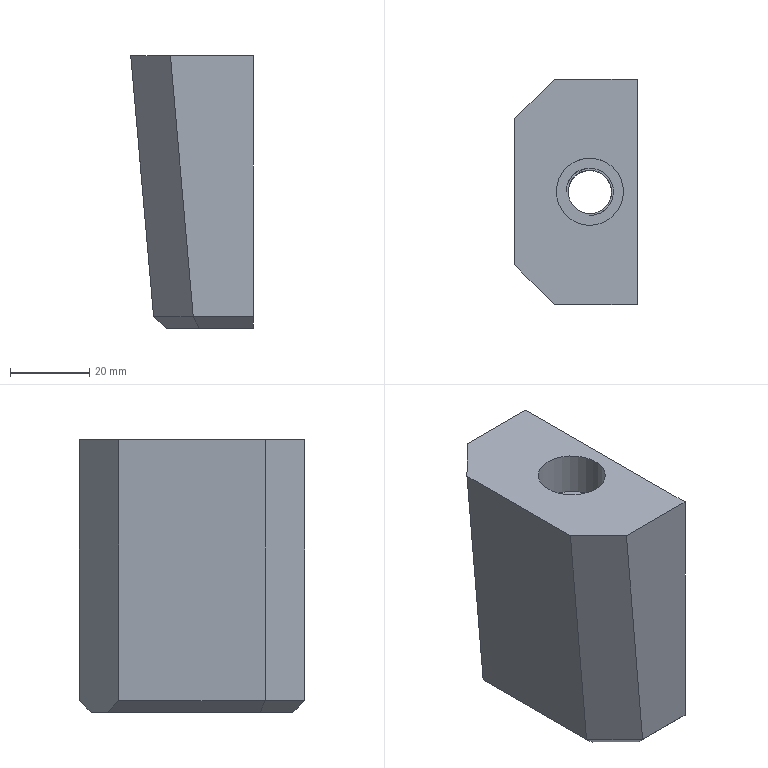Part | STEP file | P011002NM09-000 | 1 solid | 23 faces | box 31 x 57 x 69 mm | volume 94738 mm3 | plane 17 | cylinder 4 | cone 2 | commonest cylinder face diameters 11 x1 11.96 x1 12 x1 17 x1